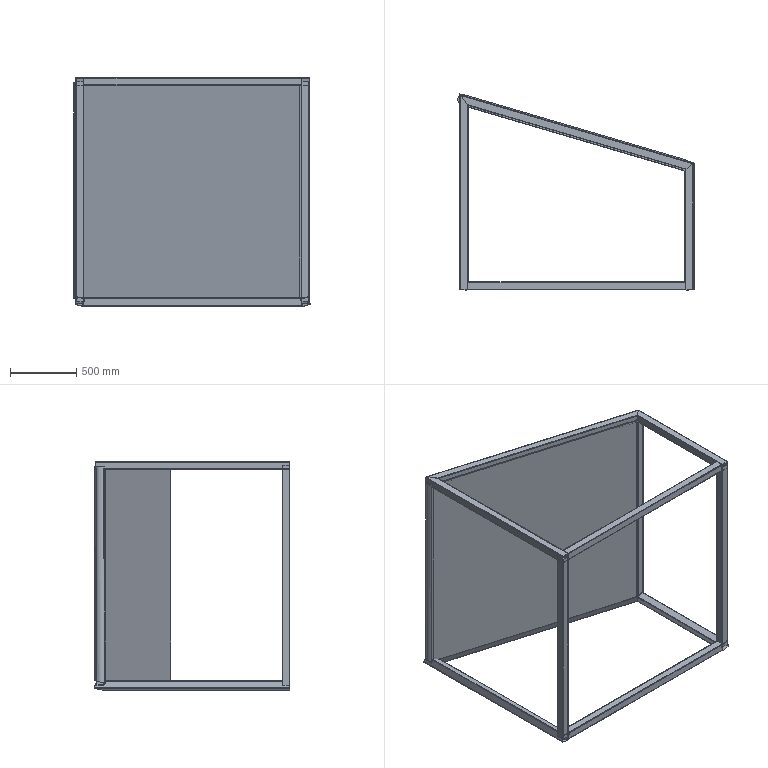Part | STEP file | Conveyor line bracket_Default<Machined> | 13 solids | 242 faces | box 1782 x 1478 x 1726 mm | volume 68319055 mm3 | plane 134 | cylinder 108 | commonest cylinder face diameters 4 x51 8 x51 60 x3 80 x3